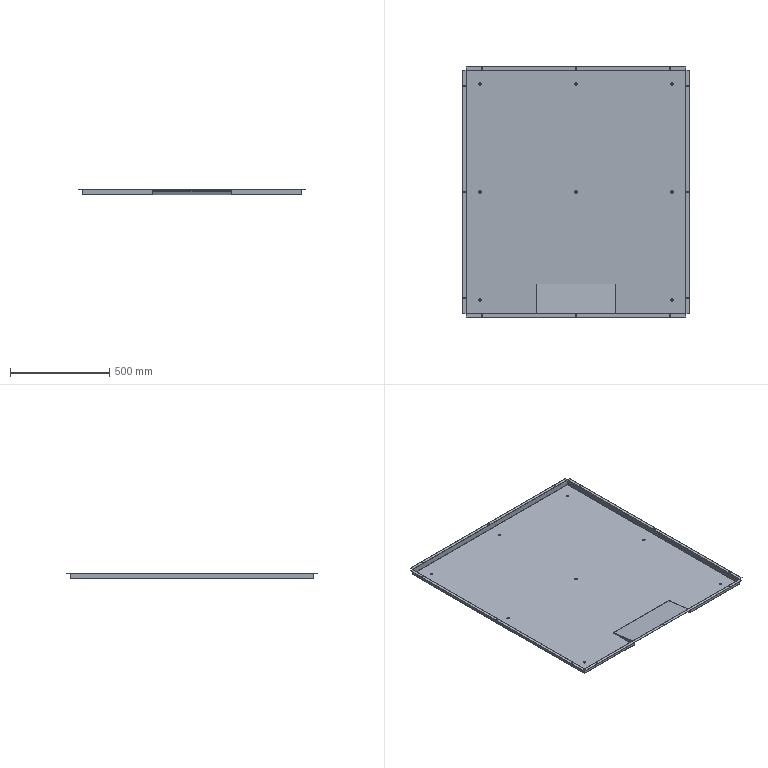Part | SolidWorks | 2 solids | 170 faces | box 1140 x 1260 x 30.147 mm | volume 1561605 mm3 | plane 90 | cylinder 68 | spline 12 | commonest cylinder face diameters 7 x30 11 x16 0.4 x9 2.4 x9 2 x2 4 x2